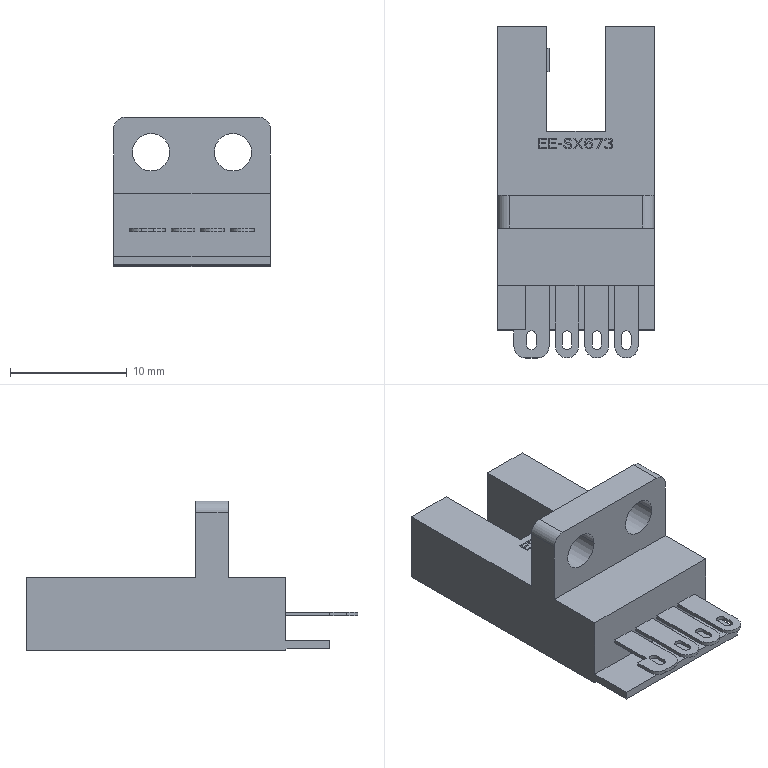Part | NX | 1 solid | 297 faces | box 13.4 x 28.4 x 12.8 mm | volume 1837 mm3 | plane 278 | cylinder 19 | commonest cylinder face diameters 0.8 x8 2 x7 3.2 x4